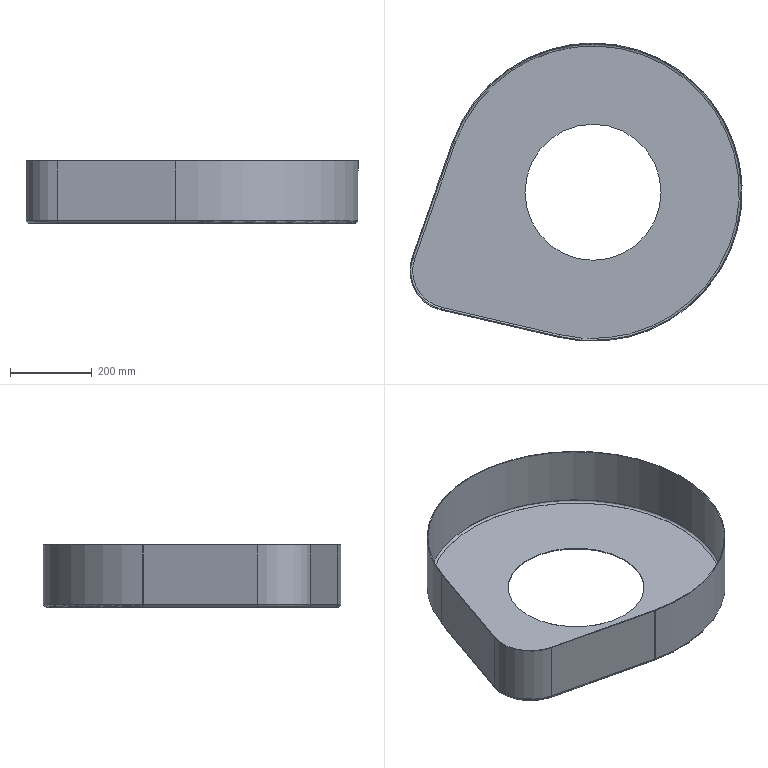Part | Creo | features DATUM PLANE 3, CURVE 2, PROTRUSION 2, ROUND 2, COORDINATE SYSTEM 1 | 1 solid | 21 faces | box 813.936 x 730.395 x 152 mm | volume 1449913 mm3 | cylinder 10 | plane 7 | torus 4 | commonest cylinder face diameters 10 x2 14 x2 333.235 x2 193.453 x1 197.453 x1 726.395 x1
STEP:
#1=CARTESIAN_POINT('',(0.,0.,0.));
#2=DIRECTION('',(0.,0.,1.));
#3=DIRECTION('',(1.,0.,0.));
#4=AXIS2_PLACEMENT_3D('',#1,#2,#3);
#5=CARTESIAN_POINT('',(-70.111,-342.323,0.));
#6=VERTEX_POINT('',#5);
#7=CARTESIAN_POINT('',(-359.981,-275.166,0.));
#8=VERTEX_POINT('',#7);
#9=CARTESIAN_POINT('',(-70.111,-342.323,0.));
#10=DIRECTION('',(-0.9742,0.2257,0.));
#11=VECTOR('',#10,297.547);
#12=LINE('',#9,#11);
#13=EDGE_CURVE('',#6,#8,#12,.T.);
#14=ORIENTED_EDGE('',*,*,#13,.F.);
#15=CARTESIAN_POINT('',(-327.227,125.326,0.));
#16=VERTEX_POINT('',#15);
#17=CARTESIAN_POINT('',(10.734,6.632,0.));
#18=DIRECTION('',(0.,0.,-1.));
#19=DIRECTION('',(-0.9435,0.3314,0.));
#20=AXIS2_PLACEMENT_3D('',#17,#18,#19);
#21=CIRCLE('',#20,358.198);
#22=EDGE_CURVE('',#16,#6,#21,.T.);
#23=ORIENTED_EDGE('',*,*,#22,.F.);
#24=CARTESIAN_POINT('',(-425.823,-155.411,0.));
#25=VERTEX_POINT('',#24);
#26=CARTESIAN_POINT('',(-425.823,-155.411,0.));
#27=DIRECTION('',(0.3314,0.9435,0.));
#28=VECTOR('',#27,297.547);
#29=LINE('',#26,#28);
#30=EDGE_CURVE('',#25,#16,#29,.T.);
#31=ORIENTED_EDGE('',*,*,#30,.F.);
#32=CARTESIAN_POINT('',(-339.278,-185.806,0.));
#33=DIRECTION('',(0.,0.,-1.));
#34=DIRECTION('',(-0.2257,-0.9742,0.));
#35=AXIS2_PLACEMENT_3D('',#32,#33,#34);
#36=CIRCLE('',#35,91.727);
#37=EDGE_CURVE('',#8,#25,#36,.T.);
#38=ORIENTED_EDGE('',*,*,#37,.F.);
#39=EDGE_LOOP('',(#14,#23,#31,#38));
#40=FACE_OUTER_BOUND('',#39,.F.);
#41=CARTESIAN_POINT('',(177.351,6.632,0.));
#42=VERTEX_POINT('',#41);
#43=CARTESIAN_POINT('',(-155.883,6.632,0.));
#44=VERTEX_POINT('',#43);
#45=CARTESIAN_POINT('',(10.734,6.632,0.));
#46=DIRECTION('',(0.,0.,-1.));
#47=DIRECTION('',(1.,0.,0.));
#48=AXIS2_PLACEMENT_3D('',#45,#46,#47);
#49=CIRCLE('',#48,166.617);
#50=EDGE_CURVE('',#42,#44,#49,.T.);
#51=ORIENTED_EDGE('',*,*,#50,.T.);
#52=CARTESIAN_POINT('',(10.734,6.632,0.));
#53=DIRECTION('',(0.,0.,-1.));
#54=DIRECTION('',(-1.,0.,0.));
#55=AXIS2_PLACEMENT_3D('',#52,#53,#54);
#56=CIRCLE('',#55,166.617);
#57=EDGE_CURVE('',#44,#42,#56,.T.);
#58=ORIENTED_EDGE('',*,*,#57,.T.);
#59=EDGE_LOOP('',(#51,#58));
#60=FACE_BOUND('',#59,.F.);
#61=CARTESIAN_POINT('',(0.,0.,0.));
#62=DIRECTION('',(0.,0.,1.));
#63=DIRECTION('',(1.,0.,0.));
#64=AXIS2_PLACEMENT_3D('',#61,#62,#63);
#65=PLANE('',#64);
#66=ADVANCED_FACE('',(#40,#60),#65,.F.);
#67=ORIENTED_EDGE('',*,*,#50,.F.);
#68=CARTESIAN_POINT('',(177.351,6.632,2.));
#69=VERTEX_POINT('',#68);
#70=CARTESIAN_POINT('',(177.351,6.632,0.));
#71=DIRECTION('',(0.,0.,1.));
#72=VECTOR('',#71,2.);
#73=LINE('',#70,#72);
#74=EDGE_CURVE('',#42,#69,#73,.T.);
#75=ORIENTED_EDGE('',*,*,#74,.T.);
#76=CARTESIAN_POINT('',(-155.883,6.632,2.));
#77=VERTEX_POINT('',#76);
#78=CARTESIAN_POINT('',(10.734,6.632,2.));
#79=DIRECTION('',(0.,0.,-1.));
#80=DIRECTION('',(1.,0.,0.));
#81=AXIS2_PLACEMENT_3D('',#78,#79,#80);
#82=CIRCLE('',#81,166.617);
#83=EDGE_CURVE('',#69,#77,#82,.T.);
#84=ORIENTED_EDGE('',*,*,#83,.T.);
#85=CARTESIAN_POINT('',(-155.883,6.632,0.));
#86=DIRECTION('',(0.,0.,1.));
#87=VECTOR('',#86,2.);
#88=LINE('',#85,#87);
#89=EDGE_CURVE('',#44,#77,#88,.T.);
#90=ORIENTED_EDGE('',*,*,#89,.F.);
#91=EDGE_LOOP('',(#67,#75,#84,#90));
#92=FACE_OUTER_BOUND('',#91,.F.);
#93=CARTESIAN_POINT('',(10.734,6.632,0.));
#94=DIRECTION('',(0.,0.,1.));
#95=DIRECTION('',(1.,0.,0.));
#96=AXIS2_PLACEMENT_3D('',#93,#94,#95);
#97=CYLINDRICAL_SURFACE('',#96,166.617);
#98=ADVANCED_FACE('',(#92),#97,.F.);
#99=ORIENTED_EDGE('',*,*,#57,.F.);
#100=ORIENTED_EDGE('',*,*,#89,.T.);
#101=CARTESIAN_POINT('',(10.734,6.632,2.));
#102=DIRECTION('',(0.,0.,-1.));
#103=DIRECTION('',(-1.,0.,0.));
#104=AXIS2_PLACEMENT_3D('',#101,#102,#103);
#105=CIRCLE('',#104,166.617);
#106=EDGE_CURVE('',#77,#69,#105,.T.);
#107=ORIENTED_EDGE('',*,*,#106,.T.);
#108=ORIENTED_EDGE('',*,*,#74,.F.);
#109=EDGE_LOOP('',(#99,#100,#107,#108));
#110=FACE_OUTER_BOUND('',#109,.F.);
#111=CARTESIAN_POINT('',(10.734,6.632,0.));
#112=DIRECTION('',(0.,0.,1.));
#113=DIRECTION('',(1.,0.,0.));
#114=AXIS2_PLACEMENT_3D('',#111,#112,#113);
#115=CYLINDRICAL_SURFACE('',#114,166.617);
#116=ADVANCED_FACE('',(#110),#115,.F.);
#117=CARTESIAN_POINT('',(-70.111,-342.323,2.));
#118=VERTEX_POINT('',#117);
#119=CARTESIAN_POINT('',(-359.981,-275.166,2.));
#120=VERTEX_POINT('',#119);
#121=CARTESIAN_POINT('',(-70.111,-342.323,2.));
#122=DIRECTION('',(-0.9742,0.2257,0.));
#123=VECTOR('',#122,297.547);
#124=LINE('',#121,#123);
#125=EDGE_CURVE('',#118,#120,#124,.T.);
#126=ORIENTED_EDGE('',*,*,#125,.T.);
#127=CARTESIAN_POINT('',(-425.823,-155.411,2.));
#128=VERTEX_POINT('',#127);
#129=CARTESIAN_POINT('',(-339.278,-185.806,2.));
#130=DIRECTION('',(0.,0.,-1.));
#131=DIRECTION('',(-0.2257,-0.9742,0.));
#132=AXIS2_PLACEMENT_3D('',#129,#130,#131);
#133=CIRCLE('',#132,91.727);
#134=EDGE_CURVE('',#120,#128,#133,.T.);
#135=ORIENTED_EDGE('',*,*,#134,.T.);
#136=CARTESIAN_POINT('',(-327.227,125.326,2.));
#137=VERTEX_POINT('',#136);
#138=CARTESIAN_POINT('',(-425.823,-155.411,2.));
#139=DIRECTION('',(0.3314,0.9435,0.));
#140=VECTOR('',#139,297.547);
#141=LINE('',#138,#140);
#142=EDGE_CURVE('',#128,#137,#141,.T.);
#143=ORIENTED_EDGE('',*,*,#142,.T.);
#144=CARTESIAN_POINT('',(10.734,6.632,2.));
#145=DIRECTION('',(0.,0.,-1.));
#146=DIRECTION('',(-0.9435,0.3314,0.));
#147=AXIS2_PLACEMENT_3D('',#144,#145,#146);
#148=CIRCLE('',#147,358.198);
#149=EDGE_CURVE('',#137,#118,#148,.T.);
#150=ORIENTED_EDGE('',*,*,#149,.T.);
#151=EDGE_LOOP('',(#126,#135,#143,#150));
#152=FACE_OUTER_BOUND('',#151,.F.);
#153=ORIENTED_EDGE('',*,*,#83,.F.);
#154=ORIENTED_EDGE('',*,*,#106,.F.);
#155=EDGE_LOOP('',(#153,#154));
#156=FACE_BOUND('',#155,.F.);
#157=CARTESIAN_POINT('',(0.,0.,2.));
#158=DIRECTION('',(0.,0.,1.));
#159=DIRECTION('',(1.,0.,0.));
#160=AXIS2_PLACEMENT_3D('',#157,#158,#159);
#161=PLANE('',#160);
#162=ADVANCED_FACE('',(#152,#156),#161,.T.);
#163=ORIENTED_EDGE('',*,*,#125,.F.);
#164=CARTESIAN_POINT('',(-71.24,-347.194,7.));
#165=VERTEX_POINT('',#164);
#166=CARTESIAN_POINT('',(-70.111,-342.323,7.));
#167=DIRECTION('',(-0.9742,0.2257,0.));
#168=DIRECTION('',(0.,0.,-1.));
#169=AXIS2_PLACEMENT_3D('',#166,#167,#168);
#170=CIRCLE('',#169,5.);
#171=EDGE_CURVE('',#118,#165,#170,.T.);
#172=ORIENTED_EDGE('',*,*,#171,.T.);
#173=CARTESIAN_POINT('',(-361.109,-280.037,7.));
#174=VERTEX_POINT('',#173);
#175=CARTESIAN_POINT('',(-71.24,-347.194,7.));
#176=DIRECTION('',(-0.9742,0.2257,0.));
#177=VECTOR('',#176,297.547);
#178=LINE('',#175,#177);
#179=EDGE_CURVE('',#165,#174,#178,.T.);
#180=ORIENTED_EDGE('',*,*,#179,.T.);
#181=CARTESIAN_POINT('',(-359.981,-275.166,7.));
#182=DIRECTION('',(-0.9742,0.2257,0.));
#183=DIRECTION('',(0.,0.,-1.));
#184=AXIS2_PLACEMENT_3D('',#181,#182,#183);
#185=CIRCLE('',#184,5.);
#186=EDGE_CURVE('',#120,#174,#185,.T.);
#187=ORIENTED_EDGE('',*,*,#186,.F.);
#188=EDGE_LOOP('',(#163,#172,#180,#187));
#189=FACE_OUTER_BOUND('',#188,.F.);
#190=CARTESIAN_POINT('',(-68.456,-342.706,7.));
#191=DIRECTION('',(-0.9742,0.2257,0.));
#192=DIRECTION('',(0.,0.,-1.));
#193=AXIS2_PLACEMENT_3D('',#190,#191,#192);
#194=CYLINDRICAL_SURFACE('',#193,5.);
#195=ADVANCED_FACE('',(#189),#194,.F.);
#196=ORIENTED_EDGE('',*,*,#149,.F.);
#197=CARTESIAN_POINT('',(-331.944,126.982,7.));
#198=VERTEX_POINT('',#197);
#199=CARTESIAN_POINT('',(-327.227,125.326,7.));
#200=DIRECTION('',(0.3314,0.9435,0.));
#201=DIRECTION('',(0.,0.,-1.));
#202=AXIS2_PLACEMENT_3D('',#199,#200,#201);
#203=CIRCLE('',#202,5.);
#204=EDGE_CURVE('',#137,#198,#203,.T.);
#205=ORIENTED_EDGE('',*,*,#204,.T.);
#206=CARTESIAN_POINT('',(10.734,6.632,7.));
#207=DIRECTION('',(0.,0.,-1.));
#208=DIRECTION('',(-0.9435,0.3314,0.));
#209=AXIS2_PLACEMENT_3D('',#206,#207,#208);
#210=CIRCLE('',#209,363.198);
#211=EDGE_CURVE('',#198,#165,#210,.T.);
#212=ORIENTED_EDGE('',*,*,#211,.T.);
#213=ORIENTED_EDGE('',*,*,#171,.F.);
#214=EDGE_LOOP('',(#196,#205,#212,#213));
#215=FACE_OUTER_BOUND('',#214,.F.);
#216=CARTESIAN_POINT('',(10.734,6.632,7.));
#217=DIRECTION('',(0.,0.,1.));
#218=DIRECTION('',(-0.9457,0.3251,0.));
#219=AXIS2_PLACEMENT_3D('',#216,#217,#218);
#220=TOROIDAL_SURFACE('',#219,358.198,5.);
#221=ADVANCED_FACE('',(#215),#220,.F.);
#222=ORIENTED_EDGE('',*,*,#142,.F.);
#223=CARTESIAN_POINT('',(-430.54,-153.755,7.));
#224=VERTEX_POINT('',#223);
#225=CARTESIAN_POINT('',(-425.823,-155.411,7.));
#226=DIRECTION('',(0.3314,0.9435,0.));
#227=DIRECTION('',(0.,0.,-1.));
#228=AXIS2_PLACEMENT_3D('',#225,#226,#227);
#229=CIRCLE('',#228,5.);
#230=EDGE_CURVE('',#128,#224,#229,.T.);
#231=ORIENTED_EDGE('',*,*,#230,.T.);
#232=CARTESIAN_POINT('',(-430.54,-153.755,7.));
#233=DIRECTION('',(0.3314,0.9435,0.));
#234=VECTOR('',#233,297.547);
#235=LINE('',#232,#234);
#236=EDGE_CURVE('',#224,#198,#235,.T.);
#237=ORIENTED_EDGE('',*,*,#236,.T.);
#238=ORIENTED_EDGE('',*,*,#204,.F.);
#239=EDGE_LOOP('',(#222,#231,#237,#238));
#240=FACE_OUTER_BOUND('',#239,.F.);
#241=CARTESIAN_POINT('',(-426.386,-157.014,7.));
#242=DIRECTION('',(0.3314,0.9435,0.));
#243=DIRECTION('',(0.,0.,-1.));
#244=AXIS2_PLACEMENT_3D('',#241,#242,#243);
#245=CYLINDRICAL_SURFACE('',#244,5.);
#246=ADVANCED_FACE('',(#240),#245,.F.);
#247=ORIENTED_EDGE('',*,*,#134,.F.);
#248=ORIENTED_EDGE('',*,*,#186,.T.);
#249=CARTESIAN_POINT('',(-339.278,-185.806,7.));
#250=DIRECTION('',(0.,0.,-1.));
#251=DIRECTION('',(-0.2257,-0.9742,0.));
#252=AXIS2_PLACEMENT_3D('',#249,#250,#251);
#253=CIRCLE('',#252,96.727);
#254=EDGE_CURVE('',#174,#224,#253,.T.);
#255=ORIENTED_EDGE('',*,*,#254,.T.);
#256=ORIENTED_EDGE('',*,*,#230,.F.);
#257=EDGE_LOOP('',(#247,#248,#255,#256));
#258=FACE_OUTER_BOUND('',#257,.F.);
#259=CARTESIAN_POINT('',(-339.278,-185.806,7.));
#260=DIRECTION('',(0.,0.,1.));
#261=DIRECTION('',(-0.2013,-0.9795,0.));
#262=AXIS2_PLACEMENT_3D('',#259,#260,#261);
#263=TOROIDAL_SURFACE('',#262,91.727,5.);
#264=ADVANCED_FACE('',(#258),#263,.F.);
#265=ORIENTED_EDGE('',*,*,#254,.F.);
#266=CARTESIAN_POINT('',(-361.109,-280.037,152.));
#267=VERTEX_POINT('',#266);
#268=CARTESIAN_POINT('',(-361.109,-280.037,7.));
#269=DIRECTION('',(0.,0.,1.));
#270=VECTOR('',#269,145.);
#271=LINE('',#268,#270);
#272=EDGE_CURVE('',#174,#267,#271,.T.);
#273=ORIENTED_EDGE('',*,*,#272,.T.);
#274=CARTESIAN_POINT('',(-430.54,-153.755,152.));
#275=VERTEX_POINT('',#274);
#276=CARTESIAN_POINT('',(-339.278,-185.806,152.));
#277=DIRECTION('',(0.,0.,-1.));
#278=DIRECTION('',(-0.2257,-0.9742,0.));
#279=AXIS2_PLACEMENT_3D('',#276,#277,#278);
#280=CIRCLE('',#279,96.727);
#281=EDGE_CURVE('',#267,#275,#280,.T.);
#282=ORIENTED_EDGE('',*,*,#281,.T.);
#283=CARTESIAN_POINT('',(-430.54,-153.755,7.));
#284=DIRECTION('',(0.,0.,1.));
#285=VECTOR('',#284,145.);
#286=LINE('',#283,#285);
#287=EDGE_CURVE('',#224,#275,#286,.T.);
#288=ORIENTED_EDGE('',*,*,#287,.F.);
#289=EDGE_LOOP('',(#265,#273,#282,#288));
#290=FACE_OUTER_BOUND('',#289,.F.);
#291=CARTESIAN_POINT('',(-339.278,-185.806,2.));
#292=DIRECTION('',(0.,0.,1.));
#293=DIRECTION('',(1.,0.,0.));
#294=AXIS2_PLACEMENT_3D('',#291,#292,#293);
#295=CYLINDRICAL_SURFACE('',#294,96.727);
#296=ADVANCED_FACE('',(#290),#295,.F.);
#297=ORIENTED_EDGE('',*,*,#179,.F.);
#298=CARTESIAN_POINT('',(-71.24,-347.194,152.));
#299=VERTEX_POINT('',#298);
#300=CARTESIAN_POINT('',(-71.24,-347.194,7.));
#301=DIRECTION('',(0.,0.,1.));
#302=VECTOR('',#301,145.);
#303=LINE('',#300,#302);
#304=EDGE_CURVE('',#165,#299,#303,.T.);
#305=ORIENTED_EDGE('',*,*,#304,.T.);
#306=CARTESIAN_POINT('',(-71.24,-347.194,152.));
#307=DIRECTION('',(-0.9742,0.2257,0.));
#308=VECTOR('',#307,297.547);
#309=LINE('',#306,#308);
#310=EDGE_CURVE('',#299,#267,#309,.T.);
#311=ORIENTED_EDGE('',*,*,#310,.T.);
#312=ORIENTED_EDGE('',*,*,#272,.F.);
#313=EDGE_LOOP('',(#297,#305,#311,#312));
#314=FACE_OUTER_BOUND('',#313,.F.);
#315=CARTESIAN_POINT('',(-71.24,-347.194,2.));
#316=DIRECTION('',(0.2257,0.9742,0.));
#317=DIRECTION('',(-0.9742,0.2257,0.));
#318=AXIS2_PLACEMENT_3D('',#315,#316,#317);
#319=PLANE('',#318);
#320=ADVANCED_FACE('',(#314),#319,.T.);
#321=ORIENTED_EDGE('',*,*,#211,.F.);
#322=CARTESIAN_POINT('',(-331.944,126.982,152.));
#323=VERTEX_POINT('',#322);
#324=CARTESIAN_POINT('',(-331.944,126.982,7.));
#325=DIRECTION('',(0.,0.,1.));
#326=VECTOR('',#325,145.);
#327=LINE('',#324,#326);
#328=EDGE_CURVE('',#198,#323,#327,.T.);
#329=ORIENTED_EDGE('',*,*,#328,.T.);
#330=CARTESIAN_POINT('',(10.734,6.632,152.));
#331=DIRECTION('',(0.,0.,-1.));
#332=DIRECTION('',(-0.9435,0.3314,0.));
#333=AXIS2_PLACEMENT_3D('',#330,#331,#332);
#334=CIRCLE('',#333,363.198);
#335=EDGE_CURVE('',#323,#299,#334,.T.);
#336=ORIENTED_EDGE('',*,*,#335,.T.);
#337=ORIENTED_EDGE('',*,*,#304,.F.);
#338=EDGE_LOOP('',(#321,#329,#336,#337));
#339=FACE_OUTER_BOUND('',#338,.F.);
#340=CARTESIAN_POINT('',(10.734,6.632,2.));
#341=DIRECTION('',(0.,0.,1.));
#342=DIRECTION('',(1.,0.,0.));
#343=AXIS2_PLACEMENT_3D('',#340,#341,#342);
#344=CYLINDRICAL_SURFACE('',#343,363.198);
#345=ADVANCED_FACE('',(#339),#344,.F.);
#346=ORIENTED_EDGE('',*,*,#236,.F.);
#347=ORIENTED_EDGE('',*,*,#287,.T.);
#348=CARTESIAN_POINT('',(-430.54,-153.755,152.));
#349=DIRECTION('',(0.3314,0.9435,0.));
#350=VECTOR('',#349,297.547);
#351=LINE('',#348,#350);
#352=EDGE_CURVE('',#275,#323,#351,.T.);
#353=ORIENTED_EDGE('',*,*,#352,.T.);
#354=ORIENTED_EDGE('',*,*,#328,.F.);
#355=EDGE_LOOP('',(#346,#347,#353,#354));
#356=FACE_OUTER_BOUND('',#355,.F.);
#357=CARTESIAN_POINT('',(-430.54,-153.755,2.));
#358=DIRECTION('',(0.9435,-0.3314,0.));
#359=DIRECTION('',(0.3314,0.9435,0.));
#360=AXIS2_PLACEMENT_3D('',#357,#358,#359);
#361=PLANE('',#360);
#362=ADVANCED_FACE('',(#356),#361,.T.);
#363=CARTESIAN_POINT('',(-71.691,-349.142,152.));
#364=VERTEX_POINT('',#363);
#365=CARTESIAN_POINT('',(-333.831,127.645,152.));
#366=VERTEX_POINT('',#365);
#367=CARTESIAN_POINT('',(10.734,6.632,152.));
#368=DIRECTION('',(0.,0.,1.));
#369=DIRECTION('',(-0.2257,-0.9742,0.));
#370=AXIS2_PLACEMENT_3D('',#367,#368,#369);
#371=CIRCLE('',#370,365.198);
#372=EDGE_CURVE('',#364,#366,#371,.T.);
#373=ORIENTED_EDGE('',*,*,#372,.F.);
#374=CARTESIAN_POINT('',(-361.561,-281.985,152.));
#375=VERTEX_POINT('',#374);
#376=CARTESIAN_POINT('',(-361.561,-281.985,152.));
#377=DIRECTION('',(0.9742,-0.2257,0.));
#378=VECTOR('',#377,297.547);
#379=LINE('',#376,#378);
#380=EDGE_CURVE('',#375,#364,#379,.T.);
#381=ORIENTED_EDGE('',*,*,#380,.F.);
#382=CARTESIAN_POINT('',(-432.427,-153.092,152.));
#383=VERTEX_POINT('',#382);
#384=CARTESIAN_POINT('',(-339.278,-185.806,152.));
#385=DIRECTION('',(0.,0.,1.));
#386=DIRECTION('',(-0.9435,0.3314,0.));
#387=AXIS2_PLACEMENT_3D('',#384,#385,#386);
#388=CIRCLE('',#387,98.727);
#389=EDGE_CURVE('',#383,#375,#388,.T.);
#390=ORIENTED_EDGE('',*,*,#389,.F.);
#391=CARTESIAN_POINT('',(-333.831,127.645,152.));
#392=DIRECTION('',(-0.3314,-0.9435,0.));
#393=VECTOR('',#392,297.547);
#394=LINE('',#391,#393);
#395=EDGE_CURVE('',#366,#383,#394,.T.);
#396=ORIENTED_EDGE('',*,*,#395,.F.);
#397=EDGE_LOOP('',(#373,#381,#390,#396));
#398=FACE_OUTER_BOUND('',#397,.F.);
#399=ORIENTED_EDGE('',*,*,#310,.F.);
#400=ORIENTED_EDGE('',*,*,#335,.F.);
#401=ORIENTED_EDGE('',*,*,#352,.F.);
#402=ORIENTED_EDGE('',*,*,#281,.F.);
#403=EDGE_LOOP('',(#399,#400,#401,#402));
#404=FACE_BOUND('',#403,.F.);
#405=CARTESIAN_POINT('',(0.,0.,152.));
#406=DIRECTION('',(0.,0.,1.));
#407=DIRECTION('',(1.,0.,0.));
#408=AXIS2_PLACEMENT_3D('',#405,#406,#407);
#409=PLANE('',#408);
#410=ADVANCED_FACE('',(#398,#404),#409,.T.);
#411=CARTESIAN_POINT('',(-333.831,127.645,7.));
#412=VERTEX_POINT('',#411);
#413=CARTESIAN_POINT('',(-71.691,-349.142,7.));
#414=VERTEX_POINT('',#413);
#415=CARTESIAN_POINT('',(10.734,6.632,7.));
#416=DIRECTION('',(0.,0.,-1.));
#417=DIRECTION('',(-0.9435,0.3314,0.));
#418=AXIS2_PLACEMENT_3D('',#415,#416,#417);
#419=CIRCLE('',#418,365.198);
#420=EDGE_CURVE('',#412,#414,#419,.T.);
#421=ORIENTED_EDGE('',*,*,#420,.T.);
#422=CARTESIAN_POINT('',(-71.691,-349.142,152.));
#423=DIRECTION('',(0.,0.,-1.));
#424=VECTOR('',#423,145.);
#425=LINE('',#422,#424);
#426=EDGE_CURVE('',#364,#414,#425,.T.);
#427=ORIENTED_EDGE('',*,*,#426,.F.);
#428=ORIENTED_EDGE('',*,*,#372,.T.);
#429=CARTESIAN_POINT('',(-333.831,127.645,7.));
#430=DIRECTION('',(0.,0.,1.));
#431=VECTOR('',#430,145.);
#432=LINE('',#429,#431);
#433=EDGE_CURVE('',#412,#366,#432,.T.);
#434=ORIENTED_EDGE('',*,*,#433,.F.);
#435=EDGE_LOOP('',(#421,#427,#428,#434));
#436=FACE_OUTER_BOUND('',#435,.F.);
#437=CARTESIAN_POINT('',(10.734,6.632,0.));
#438=DIRECTION('',(0.,0.,1.));
#439=DIRECTION('',(1.,0.,0.));
#440=AXIS2_PLACEMENT_3D('',#437,#438,#439);
#441=CYLINDRICAL_SURFACE('',#440,365.198);
#442=ADVANCED_FACE('',(#436),#441,.T.);
#443=ORIENTED_EDGE('',*,*,#22,.T.);
#444=CARTESIAN_POINT('',(-70.111,-342.323,7.));
#445=DIRECTION('',(-0.9742,0.2257,0.));
#446=DIRECTION('',(0.,0.,-1.));
#447=AXIS2_PLACEMENT_3D('',#444,#445,#446);
#448=CIRCLE('',#447,7.);
#449=EDGE_CURVE('',#6,#414,#448,.T.);
#450=ORIENTED_EDGE('',*,*,#449,.T.);
#451=ORIENTED_EDGE('',*,*,#420,.F.);
#452=CARTESIAN_POINT('',(-327.227,125.326,7.));
#453=DIRECTION('',(0.3314,0.9435,0.));
#454=DIRECTION('',(0.,0.,-1.));
#455=AXIS2_PLACEMENT_3D('',#452,#453,#454);
#456=CIRCLE('',#455,7.);
#457=EDGE_CURVE('',#16,#412,#456,.T.);
#458=ORIENTED_EDGE('',*,*,#457,.F.);
#459=EDGE_LOOP('',(#443,#450,#451,#458));
#460=FACE_OUTER_BOUND('',#459,.F.);
#461=CARTESIAN_POINT('',(10.734,6.632,7.));
#462=DIRECTION('',(0.,0.,1.));
#463=DIRECTION('',(-0.9457,0.3251,0.));
#464=AXIS2_PLACEMENT_3D('',#461,#462,#463);
#465=TOROIDAL_SURFACE('',#464,358.198,7.);
#466=ADVANCED_FACE('',(#460),#465,.T.);
#467=ORIENTED_EDGE('',*,*,#13,.T.);
#468=CARTESIAN_POINT('',(-361.561,-281.985,7.));
#469=VERTEX_POINT('',#468);
#470=CARTESIAN_POINT('',(-359.981,-275.166,7.));
#471=DIRECTION('',(-0.9742,0.2257,0.));
#472=DIRECTION('',(0.,0.,-1.));
#473=AXIS2_PLACEMENT_3D('',#470,#471,#472);
#474=CIRCLE('',#473,7.);
#475=EDGE_CURVE('',#8,#469,#474,.T.);
#476=ORIENTED_EDGE('',*,*,#475,.T.);
#477=CARTESIAN_POINT('',(-71.691,-349.142,7.));
#478=DIRECTION('',(-0.9742,0.2257,0.));
#479=VECTOR('',#478,297.547);
#480=LINE('',#477,#479);
#481=EDGE_CURVE('',#414,#469,#480,.T.);
#482=ORIENTED_EDGE('',*,*,#481,.F.);
#483=ORIENTED_EDGE('',*,*,#449,.F.);
#484=EDGE_LOOP('',(#467,#476,#482,#483));
#485=FACE_OUTER_BOUND('',#484,.F.);
#486=CARTESIAN_POINT('',(-67.76,-342.867,7.));
#487=DIRECTION('',(-0.9742,0.2257,0.));
#488=DIRECTION('',(0.,0.,-1.));
#489=AXIS2_PLACEMENT_3D('',#486,#487,#488);
#490=CYLINDRICAL_SURFACE('',#489,7.);
#491=ADVANCED_FACE('',(#485),#490,.T.);
#492=ORIENTED_EDGE('',*,*,#37,.T.);
#493=CARTESIAN_POINT('',(-432.427,-153.092,7.));
#494=VERTEX_POINT('',#493);
#495=CARTESIAN_POINT('',(-425.823,-155.411,7.));
#496=DIRECTION('',(0.3314,0.9435,0.));
#497=DIRECTION('',(0.,0.,-1.));
#498=AXIS2_PLACEMENT_3D('',#495,#496,#497);
#499=CIRCLE('',#498,7.);
#500=EDGE_CURVE('',#25,#494,#499,.T.);
#501=ORIENTED_EDGE('',*,*,#500,.T.);
#502=CARTESIAN_POINT('',(-339.278,-185.806,7.));
#503=DIRECTION('',(0.,0.,-1.));
#504=DIRECTION('',(-0.2257,-0.9742,0.));
#505=AXIS2_PLACEMENT_3D('',#502,#503,#504);
#506=CIRCLE('',#505,98.727);
#507=EDGE_CURVE('',#469,#494,#506,.T.);
#508=ORIENTED_EDGE('',*,*,#507,.F.);
#509=ORIENTED_EDGE('',*,*,#475,.F.);
#510=EDGE_LOOP('',(#492,#501,#508,#509));
#511=FACE_OUTER_BOUND('',#510,.F.);
#512=CARTESIAN_POINT('',(-339.278,-185.806,7.));
#513=DIRECTION('',(0.,0.,1.));
#514=DIRECTION('',(-0.2018,-0.9794,0.));
#515=AXIS2_PLACEMENT_3D('',#512,#513,#514);
#516=TOROIDAL_SURFACE('',#515,91.727,7.);
#517=ADVANCED_FACE('',(#511),#516,.T.);
#518=ORIENTED_EDGE('',*,*,#30,.T.);
#519=ORIENTED_EDGE('',*,*,#457,.T.);
#520=CARTESIAN_POINT('',(-432.427,-153.092,7.));
#521=DIRECTION('',(0.3314,0.9435,0.));
#522=VECTOR('',#521,297.547);
#523=LINE('',#520,#522);
#524=EDGE_CURVE('',#494,#412,#523,.T.);
#525=ORIENTED_EDGE('',*,*,#524,.F.);
#526=ORIENTED_EDGE('',*,*,#500,.F.);
#527=EDGE_LOOP('',(#518,#519,#525,#526));
#528=FACE_OUTER_BOUND('',#527,.F.);
#529=CARTESIAN_POINT('',(-426.622,-157.688,7.));
#530=DIRECTION('',(0.3314,0.9435,0.));
#531=DIRECTION('',(0.,0.,-1.));
#532=AXIS2_PLACEMENT_3D('',#529,#530,#531);
#533=CYLINDRICAL_SURFACE('',#532,7.);
#534=ADVANCED_FACE('',(#528),#533,.T.);
#535=ORIENTED_EDGE('',*,*,#524,.T.);
#536=ORIENTED_EDGE('',*,*,#433,.T.);
#537=ORIENTED_EDGE('',*,*,#395,.T.);
#538=CARTESIAN_POINT('',(-432.427,-153.092,7.));
#539=DIRECTION('',(0.,0.,1.));
#540=VECTOR('',#539,145.);
#541=LINE('',#538,#540);
#542=EDGE_CURVE('',#494,#383,#541,.T.);
#543=ORIENTED_EDGE('',*,*,#542,.F.);
#544=EDGE_LOOP('',(#535,#536,#537,#543));
#545=FACE_OUTER_BOUND('',#544,.F.);
#546=CARTESIAN_POINT('',(-333.831,127.645,0.));
#547=DIRECTION('',(-0.9435,0.3314,0.));
#548=DIRECTION('',(-0.3314,-0.9435,0.));
#549=AXIS2_PLACEMENT_3D('',#546,#547,#548);
#550=PLANE('',#549);
#551=ADVANCED_FACE('',(#545),#550,.T.);
#552=ORIENTED_EDGE('',*,*,#507,.T.);
#553=ORIENTED_EDGE('',*,*,#542,.T.);
#554=ORIENTED_EDGE('',*,*,#389,.T.);
#555=CARTESIAN_POINT('',(-361.561,-281.985,7.));
#556=DIRECTION('',(0.,0.,1.));
#557=VECTOR('',#556,145.);
#558=LINE('',#555,#557);
#559=EDGE_CURVE('',#469,#375,#558,.T.);
#560=ORIENTED_EDGE('',*,*,#559,.F.);
#561=EDGE_LOOP('',(#552,#553,#554,#560));
#562=FACE_OUTER_BOUND('',#561,.F.);
#563=CARTESIAN_POINT('',(-339.278,-185.806,0.));
#564=DIRECTION('',(0.,0.,1.));
#565=DIRECTION('',(1.,0.,0.));
#566=AXIS2_PLACEMENT_3D('',#563,#564,#565);
#567=CYLINDRICAL_SURFACE('',#566,98.727);
#568=ADVANCED_FACE('',(#562),#567,.T.);
#569=ORIENTED_EDGE('',*,*,#481,.T.);
#570=ORIENTED_EDGE('',*,*,#559,.T.);
#571=ORIENTED_EDGE('',*,*,#380,.T.);
#572=ORIENTED_EDGE('',*,*,#426,.T.);
#573=EDGE_LOOP('',(#569,#570,#571,#572));
#574=FACE_OUTER_BOUND('',#573,.F.);
#575=CARTESIAN_POINT('',(-361.561,-281.985,0.));
#576=DIRECTION('',(-0.2257,-0.9742,0.));
#577=DIRECTION('',(0.9742,-0.2257,0.));
#578=AXIS2_PLACEMENT_3D('',#575,#576,#577);
#579=PLANE('',#578);
#580=ADVANCED_FACE('',(#574),#579,.T.);
#581=CLOSED_SHELL('',(#66,#98,#116,#162,#195,#221,#246,#264,#296,#320,#345,#362,#410,#442,#466,#491,#517,#534,#551,#568,#580));
#582=MANIFOLD_SOLID_BREP('',#581);
#583=(LENGTH_UNIT()NAMED_UNIT(*)SI_UNIT(.MILLI.,.METRE.));
#584=UNCERTAINTY_MEASURE_WITH_UNIT(LENGTH_MEASURE(0.1105),#583,'','');
#585=(NAMED_UNIT(*)PLANE_ANGLE_UNIT()SI_UNIT($,.RADIAN.));
#586=PLANE_ANGLE_MEASURE_WITH_UNIT(PLANE_ANGLE_MEASURE(0.01745),#585);
#587=(CONVERSION_BASED_UNIT('DEGREE',#586)NAMED_UNIT(*)PLANE_ANGLE_UNIT());
#588=(NAMED_UNIT(*)SI_UNIT($,.STERADIAN.)SOLID_ANGLE_UNIT());
#589=(GEOMETRIC_REPRESENTATION_CONTEXT(3)GLOBAL_UNCERTAINTY_ASSIGNED_CONTEXT((#584))GLOBAL_UNIT_ASSIGNED_CONTEXT((#583,#587,#588))REPRESENTATION_CONTEXT('',''));
#590=ADVANCED_BREP_SHAPE_REPRESENTATION('',(#4,#582),#589);